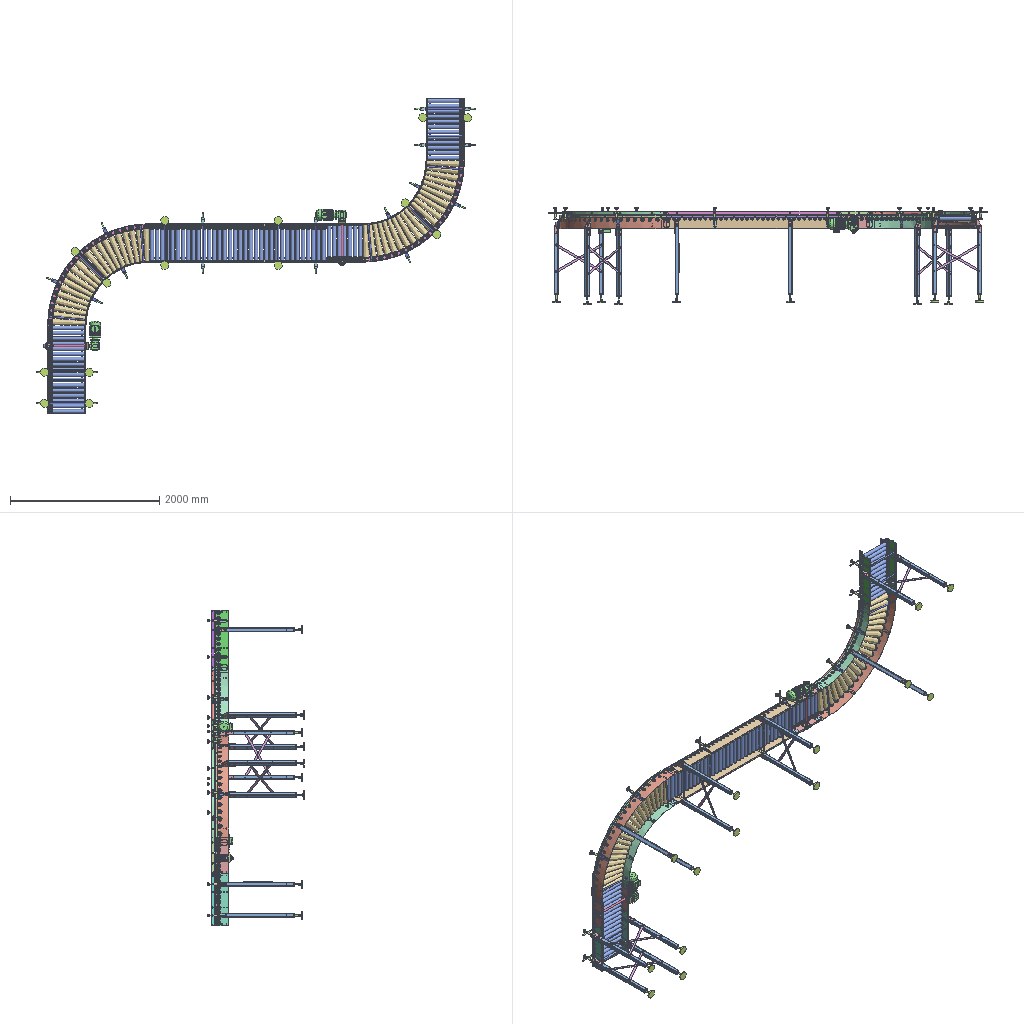Assembly | STEP file | 42 different items | 369 placed | box 5881 x 1299 x 4231 mm
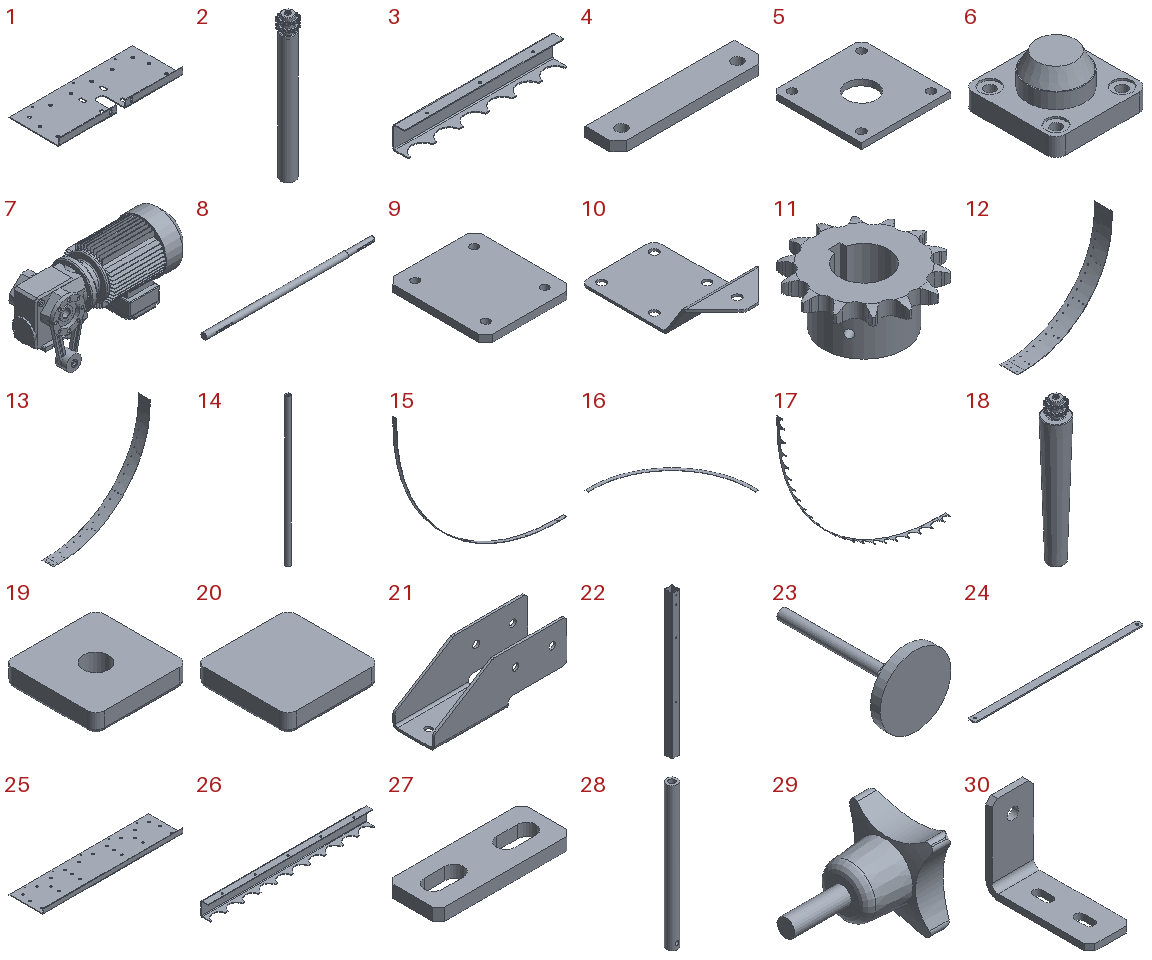Parts list (item | name | quantity | parent item | size | volume):
1 | cc-roller-motor section | x4 | in motor assembly | 418.8 x 170 x 25 mm | 188211 mm3
2 | 08b1-14 | x70 | in motor assembly, curverollers850, straight section rollers-09, straight section rollers-32, straight section rollers-10 | 63.262 x 61.879 x 506 mm | 1624253 mm3
3 | cc-coverrollers-05 | x2 | in motor assembly | 418.8 x 40 x 60 mm | 110529 mm3
4 | weldment back plate | x2 | in backplate weld | 90 x 20 x 6 mm | 10234 mm3
5 | backplate | x4 | in backplate weld, motor assembly | 90 x 90 x 6 mm | 42888 mm3
6 | 50502A | x4 | in motor assembly | 98 x 98 x 52 mm | 215908 mm3
7 | SA37TDT80N4 | x2 | in motor assembly | 398.5 x 155.5 x 203.5 mm | 5032005 mm3
8 | shaftfor roller511 | x2 | in motor assembly | 713 x 25 x 25 mm | 326518 mm3
9 | linkroller | x12 | in motor assembly, curverollers850 | 75 x 85 x 6 mm | 36985 mm3
10 | torque arm 110 | x2 | in motor assembly | 98 x 179 x 41 mm | 52160 mm3
11 | 08b1-14 | x2 | in motor assembly | 63.262 x 61.879 x 28 mm | 29059 mm3
12 | curverollersinside | x2 | in curverollers850 | 920 x 170 x 920 mm | 620259 mm3
13 | curverollersoutside | x2 | in curverollers850 | 1429 x 170 x 1429 mm | 959320 mm3
14 | axe506 | x14 | in curverollers850, straight section rollers-09, straight section rollers-32, straight section rollers-10 | 15 x 15 x 506 mm | 87993 mm3
15 | covercurveroller-p1 | x2 | in covercurveroller | 1431 x 30 x 1431 mm | 169835 mm3
16 | covercurveroller-p2 | x2 | in covercurveroller | 1428 x 1428 x 2.5 mm | 306725 mm3
17 | covercurveroller-p11 | x2 | in covercurveroller | 1374 x 60 x 1374 mm | 150099 mm3
18 | 08b1-14 | x42 | in curverollers850 | 83.871 x 83.871 x 506 mm | 1796791 mm3
19 | 14831 | x14 | in legfor roller | 50 x 50 x 10 mm | 23160 mm3
20 | 14831_CPY | x14 | in legfor roller | 50 x 50 x 10 mm | 24664 mm3
21 | Leg support-05 | x14 | in legfor roller | 180 x 56.5 x 70 mm | 69908 mm3
22 | 50x50xL-07 | x14 | in legfor roller | 50 x 50 x 900 mm | 334229 mm3
23 | 17367-articulated foot | x14 | in legfor roller | 110 x 207 x 110 mm | 212192 mm3
24 | link-forlegfor roller | x14 | in legfor roller | 725.486 x 30 x 5 mm | 107937 mm3
25 | cc-roller-09 | x2 | in straight section rollers-09 | 698 x 170 x 25 mm | 328733 mm3
26 | cc-coverrollers-09 | x1 | in straight section rollers-09 | 698 x 40 x 60 mm | 184215 mm3
27 | linkfor guide | x10 | in roller guides | 65 x 25 x 6 mm | 7799 mm3
28 | axe for guide1-02 | x20 | in guide support roller, guide support roller1 | 15 x 15 x 200 mm | 33907 mm3
29 | 13468 | x20 | in guide support roller, guide support roller1 | 57.035 x 37.729 x 37.729 mm | 20662 mm3
30 | support for guide | x12 | in guide support roller | 40 x 100 x 80 mm | 38119 mm3
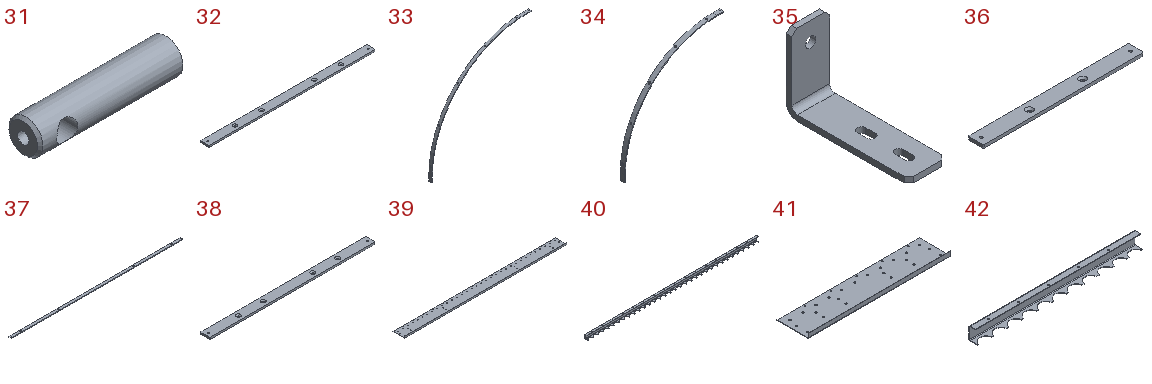31 | support1 for guide-105 | x20 | in guide support roller, guide support roller1 | 105 x 25 x 25 mm | 45078 mm3
32 | rectangular profile 40x8 | x2 | in roller guides | 767.8 x 40 x 8 mm | 241435 mm3
33 | for outer bend roller1 | x2 | in roller guides | 1382 x 40 x 1382 mm | 697130 mm3
34 | for inner bend roller | x2 | in roller guides | 938 x 40 x 938 mm | 473961 mm3
35 | support for guide1 | x8 | in guide support roller1 | 40 x 130 x 80 mm | 45319 mm3
36 | rectangular profile 40x8-419 | x4 | in roller guides | 418.8 x 40 x 8 mm | 131536 mm3
37 | rectangular profile 40x8-2303 | x2 | in roller guides | 2303 x 40 x 8 mm | 732827 mm3
38 | rectangular profile 40x8-698 | x2 | in roller guides | 698 x 40 x 8 mm | 219099 mm3
39 | cc-roller-32 | x2 | in straight section rollers-32 | 2303 x 170 x 25 mm | 1090692 mm3
40 | cc-coverrollers-32 | x1 | in straight section rollers-32 | 2303 x 40 x 60 mm | 607914 mm3
41 | cc-roller-10 | x2 | in straight section rollers-10 | 767.8 x 170 x 25 mm | 361884 mm3
42 | cc-coverrollers-10 | x1 | in straight section rollers-10 | 767.8 x 40 x 60 mm | 202679 mm3
Placements (level | parent | child | x y z in mm | rotation matrix by rows):
1 | subassembly 2 | motor assembly | -76.55 28.0 -293.364 | 1 0 0 0 1 0 0 0 1
2 | motor assembly | cc-roller-motor section | -209.4 -85.0 -12.5 | 1 0 0 0 1 0 0 0 1
2 | motor assembly | 08b1-14 | 174.5 50.0 9.104 | 1 0 0 0 -1 0 0 0 -1
2 | motor assembly | cc-roller-motor section | 209.4 -85.0 498.5 | -1 0 0 0 1 0 0 0 -1
2 | motor assembly | 08b1-14 | 104.7 50.0 9.104 | 1 0 0 0 -1 0 0 0 -1
2 | motor assembly | 08b1-14 | 34.9 50.0 9.104 | 1 0 0 0 -1 0 0 0 -1
2 | motor assembly | 08b1-14 | -34.9 50.0 9.104 | 1 0 0 0 -1 0 0 0 -1
2 | motor assembly | 08b1-14 | -104.7 50.0 9.104 | 1 0 0 0 -1 0 0 0 -1
2 | motor assembly | 08b1-14 | -174.5 50.0 9.104 | 1 0 0 0 -1 0 0 0 -1
2 | motor assembly | cc-coverrollers-05 | 209.4 65.0 -12.5 | -1 0 0 0 1 0 0 0 -1
2 | motor assembly | backplate weld | 28.767 -207.693 -38.984 | 1 0 0 0 1 0 0 0 1
3 | backplate weld | weldment back plate | -73.766 136.693 28.984 | 1 0 0 0 0 1 0 -1 0
3 | backplate weld | backplate | 126.176 142.693 28.984 | 1 0 0 0 1 0 0 0 1
2 | motor assembly | backplate | 154.943 -65.0 490.0 | 1 0 0 0 1 0 0 0 1
2 | motor assembly | 50502A | -49.0 197.629 498.5 | 1 0 0 0 1 0 0 0 1
2 | motor assembly | 50502A | 217.629 -69.0 -12.5 | 0 1 0 1 0 0 0 0 -1
2 | motor assembly | SA37TDT80N4 | -0.0 -20.0 564.5 | -1 0 0 0 0 1 0 1 -0
2 | motor assembly | shaftfor roller511 | -0.0 -20.0 653.929 | 0 0 -1 0 1 0 1 0 -0
2 | motor assembly | linkroller | -196.778 27.083 -10.0 | 1 0 0 0 1 0 0 0 1
2 | motor assembly | linkroller | -196.778 27.083 490.0 | 1 0 0 0 1 0 0 0 1
2 | motor assembly | torque arm 110 | -75.64 -116.168 498.5 | 1 0 0 0 1 0 0 0 1
2 | motor assembly | 08b1-14 | -0.0 -20.0 31.104 | 1 0 0 0 -1 0 0 0 -1
1 | subassembly 2 | curverollers850 | -123.686 119.555 202.636 | 1 0 0 0 1 0 0 0 1
2 | curverollers850 | curverollersinside | -6.975 -6.555 0.0 | 1 0 0 0 1 0 0 0 1
2 | curverollers850 | 08b1-14 | 291.536 -41.555 -486.896 | 0.3533 0.9355 0 0.9355 -0.3533 0 0 0 -1
2 | curverollers850 | 08b1-14 | 1663.433 -41.555 885.0 | 0 0 1 0 1 0 -1 0 -0
2 | curverollers850 | curverollersoutside | 142.4 -6.555 -508.5 | 1 0 0 0 1 0 0 0 1
2 | curverollers850 | axe506 | 1285.373 -146.555 -108.837 | -0.6566 -0.2625 -0.7071 0.3713 -0.9285 0 -0.6566 -0.2625 0.7071
2 | curverollers850 | axe506 | 1677.376 -146.555 731.817 | -0.02388 -0.08382 -0.9962 0.9617 -0.274 0 -0.2729 -0.9581 0.08716
2 | curverollers850 | axe506 | 444.719 -146.555 -500.84 | 0.1554 0.984 -0.08716 -0.9878 0.156 0 0.0136 0.08609 0.9962
2 | curverollers850 | covercurveroller | 1726.73 230.517 -1.54 | 0 0 -1 0 1 0 1 0 -0
3 | covercurveroller | covercurveroller-p1 | 39.985 -14.513 39.194 | 1 0 0 0 1 0 0 0 1
3 | covercurveroller | covercurveroller-p2 | 318.291 -229.571 1520.807 | 0 -1 0 0 0 1 -1 0 0
3 | covercurveroller | covercurveroller-p11 | 96.988 -44.513 96.694 | 1 0 0 0 1 0 0 0 1
2 | curverollers850 | 08b1-14 | 373.204 -58.026 -486.395 | 0.2913 -0.956 0.03489 -0.9559 -0.2923 -0.02767 0.03665 -0.02529 -0.999
2 | curverollers850 | 08b1-14 | 473.274 -58.026 -479.134 | 0.2878 -0.9514 0.1097 -0.9559 -0.2923 -0.02767 0.05839 -0.09689 -0.9936
2 | curverollers850 | 08b1-14 | 572.518 -58.026 -464.391 | 0.2826 -0.9415 0.1839 -0.9559 -0.2923 -0.02767 0.0798 -0.168 -0.9826
2 | curverollers850 | 08b1-14 | 670.377 -58.026 -442.248 | 0.2758 -0.9262 0.257 -0.9559 -0.2923 -0.02767 0.1008 -0.2381 -0.966
2 | curverollers850 | 08b1-14 | 766.3 -58.026 -412.829 | 0.2675 -0.9058 0.3287 -0.9559 -0.2923 -0.02767 0.1212 -0.3068 -0.944
2 | curverollers850 | 08b1-14 | 859.747 -58.026 -376.302 | 0.2576 -0.8802 0.3986 -0.9559 -0.2923 -0.02767 0.1409 -0.3739 -0.9167
2 | curverollers850 | 08b1-14 | 950.193 -58.026 -332.87 | 0.2463 -0.8497 0.4662 -0.9559 -0.2923 -0.02767 0.1598 -0.4388 -0.8842
2 | curverollers850 | 08b1-14 | 1037.128 -58.026 -282.78 | 0.2337 -0.8144 0.5312 -0.9559 -0.2923 -0.02767 0.1778 -0.5013 -0.8468
2 | curverollers850 | 08b1-14 | 1120.062 -58.026 -226.312 | 0.2197 -0.7745 0.5932 -0.9559 -0.2923 -0.02767 0.1948 -0.561 -0.8046
2 | curverollers850 | 08b1-14 | 1198.529 -58.026 -163.785 | 0.2045 -0.7303 0.6518 -0.9559 -0.2923 -0.02767 0.2108 -0.6175 -0.7578
2 | curverollers850 | 08b1-14 | 1272.086 -58.026 -95.55 | 0.1881 -0.6819 0.7068 -0.9559 -0.2923 -0.02767 0.2255 -0.6705 -0.7068
2 | curverollers850 | 08b1-14 | 1340.321 -58.026 -21.992 | 0.1706 -0.6297 0.7578 -0.9559 -0.2923 -0.02767 0.239 -0.7197 -0.6518
2 | curverollers850 | 08b1-14 | 1402.848 -58.026 56.474 | 0.1522 -0.574 0.8046 -0.9559 -0.2923 -0.02767 0.2511 -0.7649 -0.5932
2 | curverollers850 | 08b1-14 | 1459.316 -58.026 139.409 | 0.133 -0.515 0.8468 -0.9559 -0.2923 -0.02767 0.2618 -0.8058 -0.5312
2 | curverollers850 | 08b1-14 | 1509.407 -58.026 226.343 | 0.113 -0.4532 0.8842 -0.9559 -0.2923 -0.02767 0.271 -0.8421 -0.4662
2 | curverollers850 | 08b1-14 | 1552.838 -58.026 316.789 | 0.09234 -0.3887 0.9167 -0.9559 -0.2923 -0.02767 0.2787 -0.8737 -0.3986
2 | curverollers850 | 08b1-14 | 1589.366 -58.026 410.236 | 0.07119 -0.3221 0.944 -0.9559 -0.2923 -0.02767 0.2849 -0.9004 -0.3287
2 | curverollers850 | 08b1-14 | 1618.784 -58.026 506.159 | 0.04963 -0.2537 0.966 -0.9559 -0.2923 -0.02767 0.2894 -0.9221 -0.257
2 | curverollers850 | 08b1-14 | 1640.927 -58.026 604.018 | 0.02779 -0.1839 0.9826 -0.9559 -0.2923 -0.02767 0.2923 -0.9385 -0.1839
2 | curverollers850 | 08b1-14 | 1655.671 -58.026 703.262 | 0.005792 -0.113 0.9936 -0.9559 -0.2923 -0.02767 0.2936 -0.9496 -0.1097
2 | curverollers850 | 08b1-14 | 1662.932 -58.026 803.332 | -0.01624 -0.04146 0.999 -0.9559 -0.2923 -0.02767 0.2932 -0.9554 -0.03489
2 | curverollers850 | linkroller | 1182.536 -64.472 932.622 | 0 0 -1 0 1 0 1 0 0
2 | curverollers850 | linkroller | 1682.536 -64.472 932.622 | 0 0 -1 0 1 0 1 0 0
2 | curverollers850 | linkroller | 243.914 -168.638 -506.0 | -1 0 0 0 -1 0 0 0 1
2 | curverollers850 | linkroller | 269.159 -64.472 -6.0 | 1 0 0 0 1 0 0 0 1
1 | subassembly 2 | legfor roller | -469.367 421.023 2239.444 | 0.007492 0 1 -1 0 0.007492 0 -1 -0
2 | legfor roller | 14831 | 1367.883 487.572 1310.902 | -0.007492 0 -1 0 -1 0 -1 0 0.007492
2 | legfor roller | 14831_CPY | 450.212 487.572 1625.165 | 0.007492 0 1 0 -1 0 1 0 -0.007492
2 | legfor roller | Leg support-05 | 1845.547 603.021 1505.932 | 1 0 -0.007492 0 -1 0 -0.007492 0 -1
2 | legfor roller | 50x50xL-07 | 1359.107 636.636 1474.204 | -0.007492 0 -1 0 -1 0 -1 0 0.007492
2 | legfor roller | 17367-articulated foot | 1466.014 611.208 1463.947 | -0.007314 -1 0.001623 0.2167 0 0.9762 -0.9762 0.007492 0.2167
2 | legfor roller | Leg support-05 | 1849.375 618.895 2016.917 | 1 0 0.007492 0 1 0 -0.007492 0 1
2 | legfor roller | 14831_CPY | 454.489 764.984 2196.009 | 0 0.007492 1 1 0 0 0 1 -0.007492
2 | legfor roller | 50x50xL-07 | 1363.465 585.78 2055.931 | 0.007492 0 -1 0 1 0 1 0 0.007492
2 | legfor roller | 14831 | 1372.611 764.984 1941.852 | 0 -0.007492 -1 1 0 0 0 -1 0.007492
2 | legfor roller | 17367-articulated foot | 1470.516 611.208 2064.757 | -0.000781 -1 -0.007451 -0.9946 0 0.1042 -0.1042 0.007492 -0.9945
2 | legfor roller | link-forlegfor roller | 693.086 641.208 2075.996 | 0.4968 0.8679 0 0 0 -1 -0.8679 0.4968 -0
2 | legfor roller | link-forlegfor roller | 714.312 641.208 1448.895 | 0.5097 -0.8603 0 0 0 -1 0.8603 0.5097 -0
1 | subassembly 2 | curverollers850 | -2332.814 119.555 -303.364 | -1 0 0 0 1 0 0 0 -1
2 | curverollers850 | curverollersinside | -6.975 -6.555 0.0 | 1 0 0 0 1 0 0 0 1
2 | curverollers850 | 08b1-14 | 291.536 -41.555 -486.896 | 0.3533 0.9355 0 0.9355 -0.3533 0 0 0 -1
2 | curverollers850 | 08b1-14 | 1663.433 -41.555 885.0 | 0 0 1 0 1 0 -1 0 -0
2 | curverollers850 | curverollersoutside | 142.4 -6.555 -508.5 | 1 0 0 0 1 0 0 0 1
2 | curverollers850 | axe506 | 1285.373 -146.555 -108.837 | -0.6566 -0.2625 -0.7071 0.3713 -0.9285 0 -0.6566 -0.2625 0.7071
2 | curverollers850 | axe506 | 1677.376 -146.555 731.817 | -0.02388 -0.08382 -0.9962 0.9617 -0.274 0 -0.2729 -0.9581 0.08716
2 | curverollers850 | axe506 | 444.719 -146.555 -500.84 | 0.1554 0.984 -0.08716 -0.9878 0.156 0 0.0136 0.08609 0.9962
2 | curverollers850 | covercurveroller | 1726.73 230.517 -1.54 | 0 0 -1 0 1 0 1 0 -0
3 | covercurveroller | covercurveroller-p1 | 39.985 -14.513 39.194 | 1 0 0 0 1 0 0 0 1
3 | covercurveroller | covercurveroller-p2 | 318.291 -229.571 1520.807 | 0 -1 0 0 0 1 -1 0 0
3 | covercurveroller | covercurveroller-p11 | 96.988 -44.513 96.694 | 1 0 0 0 1 0 0 0 1
2 | curverollers850 | 08b1-14 | 373.204 -58.026 -486.395 | 0.2913 -0.956 0.03489 -0.9559 -0.2923 -0.02767 0.03665 -0.02529 -0.999
2 | curverollers850 | 08b1-14 | 473.274 -58.026 -479.134 | 0.2878 -0.9514 0.1097 -0.9559 -0.2923 -0.02767 0.05839 -0.09689 -0.9936
2 | curverollers850 | 08b1-14 | 572.518 -58.026 -464.391 | 0.2826 -0.9415 0.1839 -0.9559 -0.2923 -0.02767 0.0798 -0.168 -0.9826
2 | curverollers850 | 08b1-14 | 670.377 -58.026 -442.248 | 0.2758 -0.9262 0.257 -0.9559 -0.2923 -0.02767 0.1008 -0.2381 -0.966
2 | curverollers850 | 08b1-14 | 766.3 -58.026 -412.829 | 0.2675 -0.9058 0.3287 -0.9559 -0.2923 -0.02767 0.1212 -0.3068 -0.944
2 | curverollers850 | 08b1-14 | 859.747 -58.026 -376.302 | 0.2576 -0.8802 0.3986 -0.9559 -0.2923 -0.02767 0.1409 -0.3739 -0.9167
2 | curverollers850 | 08b1-14 | 950.193 -58.026 -332.87 | 0.2463 -0.8497 0.4662 -0.9559 -0.2923 -0.02767 0.1598 -0.4388 -0.8842
2 | curverollers850 | 08b1-14 | 1037.128 -58.026 -282.78 | 0.2337 -0.8144 0.5312 -0.9559 -0.2923 -0.02767 0.1778 -0.5013 -0.8468
2 | curverollers850 | 08b1-14 | 1120.062 -58.026 -226.312 | 0.2197 -0.7745 0.5932 -0.9559 -0.2923 -0.02767 0.1948 -0.561 -0.8046
2 | curverollers850 | 08b1-14 | 1198.529 -58.026 -163.785 | 0.2045 -0.7303 0.6518 -0.9559 -0.2923 -0.02767 0.2108 -0.6175 -0.7578
2 | curverollers850 | 08b1-14 | 1272.086 -58.026 -95.55 | 0.1881 -0.6819 0.7068 -0.9559 -0.2923 -0.02767 0.2255 -0.6705 -0.7068
2 | curverollers850 | 08b1-14 | 1340.321 -58.026 -21.992 | 0.1706 -0.6297 0.7578 -0.9559 -0.2923 -0.02767 0.239 -0.7197 -0.6518
2 | curverollers850 | 08b1-14 | 1402.848 -58.026 56.474 | 0.1522 -0.574 0.8046 -0.9559 -0.2923 -0.02767 0.2511 -0.7649 -0.5932
2 | curverollers850 | 08b1-14 | 1459.316 -58.026 139.409 | 0.133 -0.515 0.8468 -0.9559 -0.2923 -0.02767 0.2618 -0.8058 -0.5312
2 | curverollers850 | 08b1-14 | 1509.407 -58.026 226.343 | 0.113 -0.4532 0.8842 -0.9559 -0.2923 -0.02767 0.271 -0.8421 -0.4662
2 | curverollers850 | 08b1-14 | 1552.838 -58.026 316.789 | 0.09234 -0.3887 0.9167 -0.9559 -0.2923 -0.02767 0.2787 -0.8737 -0.3986
2 | curverollers850 | 08b1-14 | 1589.366 -58.026 410.236 | 0.07119 -0.3221 0.944 -0.9559 -0.2923 -0.02767 0.2849 -0.9004 -0.3287
2 | curverollers850 | 08b1-14 | 1618.784 -58.026 506.159 | 0.04963 -0.2537 0.966 -0.9559 -0.2923 -0.02767 0.2894 -0.9221 -0.257
2 | curverollers850 | 08b1-14 | 1640.927 -58.026 604.018 | 0.02779 -0.1839 0.9826 -0.9559 -0.2923 -0.02767 0.2923 -0.9385 -0.1839
2 | curverollers850 | 08b1-14 | 1655.671 -58.026 703.262 | 0.005792 -0.113 0.9936 -0.9559 -0.2923 -0.02767 0.2936 -0.9496 -0.1097
2 | curverollers850 | 08b1-14 | 1662.932 -58.026 803.332 | -0.01624 -0.04146 0.999 -0.9559 -0.2923 -0.02767 0.2932 -0.9554 -0.03489
2 | curverollers850 | linkroller | 1182.536 -64.472 932.622 | 0 0 -1 0 1 0 1 0 0
2 | curverollers850 | linkroller | 1682.536 -64.472 932.622 | 0 0 -1 0 1 0 1 0 0
2 | curverollers850 | linkroller | 243.914 -168.638 -506.0 | -1 0 0 0 -1 0 0 0 1
2 | curverollers850 | linkroller | 269.159 -64.472 -6.0 | 1 0 0 0 1 0 0 0 1
1 | subassembly 2 | motor assembly | -4005.35 28.0 -1432.764 | 0 0 1 0 1 0 -1 0 0
2 | motor assembly | cc-roller-motor section | -209.4 -85.0 -12.5 | 1 0 0 0 1 0 0 0 1
2 | motor assembly | 08b1-14 | 174.5 50.0 9.104 | 1 0 0 0 -1 0 0 0 -1
2 | motor assembly | cc-roller-motor section | 209.4 -85.0 498.5 | -1 0 0 0 1 0 0 0 -1
2 | motor assembly | 08b1-14 | 104.7 50.0 9.104 | 1 0 0 0 -1 0 0 0 -1
2 | motor assembly | 08b1-14 | 34.9 50.0 9.104 | 1 0 0 0 -1 0 0 0 -1
2 | motor assembly | 08b1-14 | -34.9 50.0 9.104 | 1 0 0 0 -1 0 0 0 -1
2 | motor assembly | 08b1-14 | -104.7 50.0 9.104 | 1 0 0 0 -1 0 0 0 -1
2 | motor assembly | 08b1-14 | -174.5 50.0 9.104 | 1 0 0 0 -1 0 0 0 -1
2 | motor assembly | cc-coverrollers-05 | 209.4 65.0 -12.5 | -1 0 0 0 1 0 0 0 -1
2 | motor assembly | backplate weld | 28.767 -207.693 -38.984 | 1 0 0 0 1 0 0 0 1
3 | backplate weld | weldment back plate | -73.766 136.693 28.984 | 1 0 0 0 0 1 0 -1 0
3 | backplate weld | backplate | 126.176 142.693 28.984 | 1 0 0 0 1 0 0 0 1
2 | motor assembly | backplate | 154.943 -65.0 490.0 | 1 0 0 0 1 0 0 0 1
2 | motor assembly | 50502A | -49.0 197.629 498.5 | 1 0 0 0 1 0 0 0 1
2 | motor assembly | 50502A | 217.629 -69.0 -12.5 | 0 1 0 1 0 0 0 0 -1
2 | motor assembly | SA37TDT80N4 | -0.0 -20.0 564.5 | -1 0 0 0 0 1 0 1 -0
2 | motor assembly | shaftfor roller511 | -0.0 -20.0 653.929 | 0 0 -1 0 1 0 1 0 -0
2 | motor assembly | linkroller | -196.778 27.083 -10.0 | 1 0 0 0 1 0 0 0 1
2 | motor assembly | linkroller | -196.778 27.083 490.0 | 1 0 0 0 1 0 0 0 1
2 | motor assembly | torque arm 110 | -75.64 -116.168 498.5 | 1 0 0 0 1 0 0 0 1
2 | motor assembly | 08b1-14 | -0.0 -20.0 31.104 | 1 0 0 0 -1 0 0 0 -1
1 | subassembly 2 | straight section rollers-09 | -4270.85 -64.5 -1634.664 | 0 0 1 0 1 0 -1 0 -0
2 | straight section rollers-09 | axe506 | 565.5 27.5 255.5 | 1 0 0 0 1 0 0 0 1
2 | straight section rollers-09 | cc-roller-09 | 7.5 7.5 253.0 | 1 0 0 0 1 0 0 0 1
2 | straight section rollers-09 | cc-coverrollers-09 | 705.5 157.5 253.0 | -1 0 0 0 1 0 0 0 -1
2 | straight section rollers-09 | cc-roller-09 | 705.5 7.5 764.0 | -1 0 0 0 1 0 0 0 -1
2 | straight section rollers-09 | 08b1-14 | 670.6 142.5 274.604 | 1 0 0 0 -1 0 0 0 -1
2 | straight section rollers-09 | 08b1-14 | 600.8 142.5 274.604 | 1 0 0 0 -1 0 0 0 -1
2 | straight section rollers-09 | 08b1-14 | 531.0 142.5 274.604 | 1 0 0 0 -1 0 0 0 -1
2 | straight section rollers-09 | 08b1-14 | 461.2 142.5 274.604 | 1 0 0 0 -1 0 0 0 -1
2 | straight section rollers-09 | 08b1-14 | 391.4 142.5 274.604 | 1 0 0 0 -1 0 0 0 -1
2 | straight section rollers-09 | 08b1-14 | 321.6 142.5 274.604 | 1 0 0 0 -1 0 0 0 -1
2 | straight section rollers-09 | 08b1-14 | 251.8 142.5 274.604 | 1 0 0 0 -1 0 0 0 -1
2 | straight section rollers-09 | 08b1-14 | 182.0 142.5 274.604 | 1 0 0 0 -1 0 0 0 -1
2 | straight section rollers-09 | 08b1-14 | 112.2 142.5 274.604 | 1 0 0 0 -1 0 0 0 -1
2 | straight section rollers-09 | 08b1-14 | 42.4 142.5 274.604 | 1 0 0 0 -1 0 0 0 -1
2 | straight section rollers-09 | axe506 | 252.0 27.5 255.5 | 1 0 0 0 1 0 0 0 1
1 | subassembly 2 | legfor roller | -1987.133 421.023 -2811.122 | -0.007492 0 -1 -1 0 0.007492 0 1 0
2 | legfor roller | 14831 | 1367.883 487.572 1310.902 | -0.007492 0 -1 0 -1 0 -1 0 0.007492
2 | legfor roller | 14831_CPY | 450.212 487.572 1625.165 | 0.007492 0 1 0 -1 0 1 0 -0.007492
2 | legfor roller | Leg support-05 | 1845.547 603.021 1505.932 | 1 0 -0.007492 0 -1 0 -0.007492 0 -1
2 | legfor roller | 50x50xL-07 | 1359.107 636.636 1474.204 | -0.007492 0 -1 0 -1 0 -1 0 0.007492
2 | legfor roller | 17367-articulated foot | 1466.014 611.208 1463.947 | -0.007314 -1 0.001623 0.2167 0 0.9762 -0.9762 0.007492 0.2167
2 | legfor roller | Leg support-05 | 1849.375 618.895 2016.917 | 1 0 0.007492 0 1 0 -0.007492 0 1
2 | legfor roller | 14831_CPY | 454.489 764.984 2196.009 | 0 0.007492 1 1 0 0 0 1 -0.007492
2 | legfor roller | 50x50xL-07 | 1363.465 585.78 2055.931 | 0.007492 0 -1 0 1 0 1 0 0.007492
2 | legfor roller | 14831 | 1372.611 764.984 1941.852 | 0 -0.007492 -1 1 0 0 0 -1 0.007492
2 | legfor roller | 17367-articulated foot | 1470.516 611.208 2064.757 | -0.000781 -1 -0.007451 -0.9946 0 0.1042 -0.1042 0.007492 -0.9945
2 | legfor roller | link-forlegfor roller | 693.086 641.208 2075.996 | 0.4968 0.8679 0 0 0 -1 -0.8679 0.4968 -0
2 | legfor roller | link-forlegfor roller | 714.312 641.208 1448.895 | 0.5097 -0.8603 0 0 0 -1 0.8603 0.5097 -0
1 | subassembly 2 | legfor roller | 1806.044 391.024 -1414.582 | -0.005298 0.7071 -0.7071 -1 0 0.007492 0.005298 0.7071 0.7071
2 | legfor roller | 14831 | 1367.883 487.572 1310.902 | -0.007492 0 -1 0 -1 0 -1 0 0.007492
2 | legfor roller | 14831_CPY | 450.212 487.572 1625.165 | 0.007492 0 1 0 -1 0 1 0 -0.007492
2 | legfor roller | Leg support-05 | 1845.547 603.021 1505.932 | 1 0 -0.007492 0 -1 0 -0.007492 0 -1
2 | legfor roller | 50x50xL-07 | 1359.107 636.636 1474.204 | -0.007492 0 -1 0 -1 0 -1 0 0.007492
2 | legfor roller | 17367-articulated foot | 1466.014 611.208 1463.947 | -0.007314 -1 0.001623 0.2167 0 0.9762 -0.9762 0.007492 0.2167
2 | legfor roller | Leg support-05 | 1849.375 618.895 2016.917 | 1 0 0.007492 0 1 0 -0.007492 0 1
2 | legfor roller | 14831_CPY | 454.489 764.984 2196.009 | 0 0.007492 1 1 0 0 0 1 -0.007492
2 | legfor roller | 50x50xL-07 | 1363.465 585.78 2055.931 | 0.007492 0 -1 0 1 0 1 0 0.007492
2 | legfor roller | 14831 | 1372.611 764.984 1941.852 | 0 -0.007492 -1 1 0 0 0 -1 0.007492
2 | legfor roller | 17367-articulated foot | 1470.516 611.208 2064.757 | -0.000781 -1 -0.007451 -0.9946 0 0.1042 -0.1042 0.007492 -0.9945
2 | legfor roller | link-forlegfor roller | 693.086 641.208 2075.996 | 0.4968 0.8679 0 0 0 -1 -0.8679 0.4968 -0
2 | legfor roller | link-forlegfor roller | 714.312 641.208 1448.895 | 0.5097 -0.8603 0 0 0 -1 0.8603 0.5097 -0
1 | subassembly 2 | legfor roller | -1542.758 421.023 -1825.58 | 0 1 0 -1 0 0.007492 0.007492 0 1
2 | legfor roller | 14831 | 1367.883 487.572 1310.902 | -0.007492 0 -1 0 -1 0 -1 0 0.007492
2 | legfor roller | 14831_CPY | 450.212 487.572 1625.165 | 0.007492 0 1 0 -1 0 1 0 -0.007492
2 | legfor roller | Leg support-05 | 1845.547 603.021 1505.932 | 1 0 -0.007492 0 -1 0 -0.007492 0 -1
2 | legfor roller | 50x50xL-07 | 1359.107 636.636 1474.204 | -0.007492 0 -1 0 -1 0 -1 0 0.007492
2 | legfor roller | 17367-articulated foot | 1466.014 611.208 1463.947 | -0.007314 -1 0.001623 0.2167 0 0.9762 -0.9762 0.007492 0.2167
2 | legfor roller | Leg support-05 | 1849.375 618.895 2016.917 | 1 0 0.007492 0 1 0 -0.007492 0 1
2 | legfor roller | 14831_CPY | 454.489 764.984 2196.009 | 0 0.007492 1 1 0 0 0 1 -0.007492
2 | legfor roller | 50x50xL-07 | 1363.465 585.78 2055.931 | 0.007492 0 -1 0 1 0 1 0 0.007492
2 | legfor roller | 14831 | 1372.611 764.984 1941.852 | 0 -0.007492 -1 1 0 0 0 -1 0.007492
2 | legfor roller | 17367-articulated foot | 1470.516 611.208 2064.757 | -0.000781 -1 -0.007451 -0.9946 0 0.1042 -0.1042 0.007492 -0.9945
2 | legfor roller | link-forlegfor roller | 693.086 641.208 2075.996 | 0.4968 0.8679 0 0 0 -1 -0.8679 0.4968 -0
2 | legfor roller | link-forlegfor roller | 714.312 641.208 1448.895 | 0.5097 -0.8603 0 0 0 -1 0.8603 0.5097 -0
1 | subassembly 2 | legfor roller | -2616.034 391.023 -2060.705 | -0.005298 0.7071 -0.7071 -1 0 0.007492 0.005298 0.7071 0.7071
2 | legfor roller | 14831 | 1367.883 487.572 1310.902 | -0.007492 0 -1 0 -1 0 -1 0 0.007492
2 | legfor roller | 14831_CPY | 450.212 487.572 1625.165 | 0.007492 0 1 0 -1 0 1 0 -0.007492
2 | legfor roller | Leg support-05 | 1845.547 603.021 1505.932 | 1 0 -0.007492 0 -1 0 -0.007492 0 -1
2 | legfor roller | 50x50xL-07 | 1359.107 636.636 1474.204 | -0.007492 0 -1 0 -1 0 -1 0 0.007492
2 | legfor roller | 17367-articulated foot | 1466.014 611.208 1463.947 | -0.007314 -1 0.001623 0.2167 0 0.9762 -0.9762 0.007492 0.2167
2 | legfor roller | Leg support-05 | 1849.375 618.895 2016.917 | 1 0 0.007492 0 1 0 -0.007492 0 1
2 | legfor roller | 14831_CPY | 454.489 764.984 2196.009 | 0 0.007492 1 1 0 0 0 1 -0.007492
2 | legfor roller | 50x50xL-07 | 1363.465 585.78 2055.931 | 0.007492 0 -1 0 1 0 1 0 0.007492
2 | legfor roller | 14831 | 1372.611 764.984 1941.852 | 0 -0.007492 -1 1 0 0 0 -1 0.007492
2 | legfor roller | 17367-articulated foot | 1470.516 611.208 2064.757 | -0.000781 -1 -0.007451 -0.9946 0 0.1042 -0.1042 0.007492 -0.9945
2 | legfor roller | link-forlegfor roller | 693.086 641.208 2075.996 | 0.4968 0.8679 0 0 0 -1 -0.8679 0.4968 -0
2 | legfor roller | link-forlegfor roller | 714.312 641.208 1448.895 | 0.5097 -0.8603 0 0 0 -1 0.8603 0.5097 -0
1 | subassembly 2 | legfor roller | -1987.133 421.023 -2393.122 | -0.007492 0 -1 -1 0 0.007492 0 1 0
2 | legfor roller | 14831 | 1367.883 487.572 1310.902 | -0.007492 0 -1 0 -1 0 -1 0 0.007492
2 | legfor roller | 14831_CPY | 450.212 487.572 1625.165 | 0.007492 0 1 0 -1 0 1 0 -0.007492
2 | legfor roller | Leg support-05 | 1845.547 603.021 1505.932 | 1 0 -0.007492 0 -1 0 -0.007492 0 -1
2 | legfor roller | 50x50xL-07 | 1359.107 636.636 1474.204 | -0.007492 0 -1 0 -1 0 -1 0 0.007492
2 | legfor roller | 17367-articulated foot | 1466.014 611.208 1463.947 | -0.007314 -1 0.001623 0.2167 0 0.9762 -0.9762 0.007492 0.2167
2 | legfor roller | Leg support-05 | 1849.375 618.895 2016.917 | 1 0 0.007492 0 1 0 -0.007492 0 1
2 | legfor roller | 14831_CPY | 454.489 764.984 2196.009 | 0 0.007492 1 1 0 0 0 1 -0.007492
2 | legfor roller | 50x50xL-07 | 1363.465 585.78 2055.931 | 0.007492 0 -1 0 1 0 1 0 0.007492
2 | legfor roller | 14831 | 1372.611 764.984 1941.852 | 0 -0.007492 -1 1 0 0 0 -1 0.007492
2 | legfor roller | 17367-articulated foot | 1470.516 611.208 2064.757 | -0.000781 -1 -0.007451 -0.9946 0 0.1042 -0.1042 0.007492 -0.9945
2 | legfor roller | link-forlegfor roller | 693.086 641.208 2075.996 | 0.4968 0.8679 0 0 0 -1 -0.8679 0.4968 -0
2 | legfor roller | link-forlegfor roller | 714.312 641.208 1448.895 | 0.5097 -0.8603 0 0 0 -1 0.8603 0.5097 -0
1 | subassembly 2 | linkfor guide | -3549.854 163.846 -931.057 | 0 0 -1 0 1 0 1 0 -0
1 | subassembly 2 | linkfor guide | -3974.846 163.846 -866.057 | 0 0 1 0 1 0 -1 0 0
1 | subassembly 2 | roller guides | -1448.011 -1380.613 425.582 | 1 0 0 0 1 0 0 0 1
2 | roller guides | guide support roller | 3085.357 1538.613 837.054 | 0 0 -1 -0.5657 -0.8246 0 -0.8246 0.5657 0
3 | guide support roller | axe for guide1-02 | 0.0 0.0 -75.0 | 1 0 0 0 1 0 0 0 1
3 | guide support roller | 13468 | -19.942 28.405 15.996 | -0.5657 0.8246 0 -0.8246 -0.5657 0 0 0 1
3 | guide support roller | support for guide | 40.212 106.981 75.996 | 0.8246 -0.5657 0 -0.5657 -0.8246 0 0 0 -1
3 | guide support roller | support1 for guide-105 | -15.089 -21.994 13.53 | 0.5657 0 0.8246 0.8246 0 -0.5657 0 1 -0
2 | roller guides | guide support roller | 3085.357 1538.613 1324.854 | 0 0 -1 -0.5657 -0.8246 0 -0.8246 0.5657 0
3 | guide support roller | axe for guide1-02 | 0.0 0.0 -75.0 | 1 0 0 0 1 0 0 0 1
3 | guide support roller | 13468 | -19.942 28.405 15.996 | -0.5657 0.8246 0 -0.8246 -0.5657 0 0 0 1
3 | guide support roller | support for guide | 40.212 106.981 75.996 | 0.8246 -0.5657 0 -0.5657 -0.8246 0 0 0 -1
3 | guide support roller | support1 for guide-105 | -15.089 -21.994 13.53 | 0.5657 0 0.8246 0.8246 0 -0.5657 0 1 -0
2 | roller guides | guide support roller | 2422.365 1538.613 1324.854 | 0 0 1 -0.5657 -0.8246 0 0.8246 -0.5657 -0
3 | guide support roller | axe for guide1-02 | 0.0 0.0 -75.0 | 1 0 0 0 1 0 0 0 1
3 | guide support roller | 13468 | -19.942 28.405 15.996 | -0.5657 0.8246 0 -0.8246 -0.5657 0 0 0 1
3 | guide support roller | support for guide | 40.212 106.981 75.996 | 0.8246 -0.5657 0 -0.5657 -0.8246 0 0 0 -1
3 | guide support roller | support1 for guide-105 | -15.089 -21.994 13.53 | 0.5657 0 0.8246 0.8246 0 -0.5657 0 1 -0
2 | roller guides | rectangular profile 40x8 | 2547.365 1772.801 1464.854 | 0 0 1 0 1 0 -1 0 -0
2 | roller guides | guide support roller | 2422.365 1538.613 837.054 | 0 0 1 -0.5657 -0.8246 0 0.8246 -0.5657 -0
3 | guide support roller | axe for guide1-02 | 0.0 0.0 -75.0 | 1 0 0 0 1 0 0 0 1
3 | guide support roller | 13468 | -19.942 28.405 15.996 | -0.5657 0.8246 0 -0.8246 -0.5657 0 0 0 1
3 | guide support roller | support for guide | 40.212 106.981 75.996 | 0.8246 -0.5657 0 -0.5657 -0.8246 0 0 0 -1
3 | guide support roller | support1 for guide-105 | -15.089 -21.994 13.53 | 0.5657 0 0.8246 0.8246 0 -0.5657 0 1 -0
2 | roller guides | rectangular profile 40x8 | 2960.357 1772.801 697.054 | 0 0 -1 0 1 0 1 0 0
2 | roller guides | for outer bend roller1 | 2969.861 1413.685 432.302 | 0 0 1 0 -1 0 1 0 -0
2 | roller guides | for inner bend roller | 2525.861 1413.685 242.01 | 0 0 1 0 -1 0 1 0 -0
2 | roller guides | guide support roller1 | 2950.956 1538.613 20.81 | -0.3485 0.2391 -0.9063 -0.5657 -0.8246 0 -0.7473 0.5127 0.4226
3 | guide support roller1 | axe for guide1-02 | -0.0 0.0 -75.0 | 1 0 0 0 1 0 0 0 1
3 | guide support roller1 | 13468 | -19.942 28.405 15.996 | -0.5657 0.8246 0 -0.8246 -0.5657 0 0 0 1
3 | guide support roller1 | support for guide1 | 40.212 106.981 75.996 | 0.8246 -0.5657 0 -0.5657 -0.8246 0 0 0 -1
3 | guide support roller1 | support1 for guide-105 | -15.089 -21.994 13.53 | 0.5657 0 0.8246 0.8246 0 -0.5657 0 1 -0
2 | roller guides | guide support roller1 | 2350.081 1538.613 301.002 | 0.3485 -0.2391 0.9063 -0.5657 -0.8246 0 0.7473 -0.5127 -0.4226
3 | guide support roller1 | axe for guide1-02 | -0.0 0.0 -75.0 | 1 0 0 0 1 0 0 0 1
3 | guide support roller1 | 13468 | -19.942 28.405 15.996 | -0.5657 0.8246 0 -0.8246 -0.5657 0 0 0 1
3 | guide support roller1 | support for guide1 | 40.212 106.981 75.996 | 0.8246 -0.5657 0 -0.5657 -0.8246 0 0 0 -1
3 | guide support roller1 | support1 for guide-105 | -15.089 -21.994 13.53 | 0.5657 0 0.8246 0.8246 0 -0.5657 0 1 -0
2 | roller guides | guide support roller1 | 1976.913 1538.613 -72.166 | 0.7473 -0.5127 0.4226 -0.5657 -0.8246 0 0.3485 -0.2391 -0.9063
3 | guide support roller1 | axe for guide1-02 | -0.0 0.0 -75.0 | 1 0 0 0 1 0 0 0 1
3 | guide support roller1 | 13468 | -19.942 28.405 15.996 | -0.5657 0.8246 0 -0.8246 -0.5657 0 0 0 1
3 | guide support roller1 | support for guide1 | 40.212 106.981 75.996 | 0.8246 -0.5657 0 -0.5657 -0.8246 0 0 0 -1
3 | guide support roller1 | support1 for guide-105 | -15.089 -21.994 13.53 | 0.5657 0 0.8246 0.8246 0 -0.5657 0 1 -0
2 | roller guides | guide support roller1 | 2257.105 1538.613 -673.041 | -0.7473 0.5127 -0.4226 -0.5657 -0.8246 0 -0.3485 0.2391 0.9063
3 | guide support roller1 | axe for guide1-02 | -0.0 0.0 -75.0 | 1 0 0 0 1 0 0 0 1
3 | guide support roller1 | 13468 | -19.942 28.405 15.996 | -0.5657 0.8246 0 -0.8246 -0.5657 0 0 0 1
3 | guide support roller1 | support for guide1 | 40.212 106.981 75.996 | 0.8246 -0.5657 0 -0.5657 -0.8246 0 0 0 -1
3 | guide support roller1 | support1 for guide-105 | -15.089 -21.994 13.53 | 0.5657 0 0.8246 0.8246 0 -0.5657 0 1 -0
2 | roller guides | linkfor guide | 1555.861 1544.459 -688.442 | 1 0 0 0 1 0 0 0 1
2 | roller guides | linkfor guide | 1555.861 1544.459 -269.45 | 1 0 0 0 1 0 0 0 1
2 | roller guides | rectangular profile 40x8-419 | 1580.861 1772.801 -269.45 | -1 0 0 0 1 0 0 0 -1
2 | roller guides | linkfor guide | 1137.061 1544.459 -688.442 | 1 0 0 0 1 0 0 0 1
2 | roller guides | rectangular profile 40x8-419 | 1162.061 1772.801 -682.442 | 1 0 0 0 1 0 0 0 1
2 | roller guides | rectangular profile 40x8-2303 | -1141.339 1772.801 -682.442 | 1 0 0 0 1 0 0 0 1
2 | roller guides | linkfor guide | 1137.061 1544.459 -269.45 | 1 0 0 0 1 0 0 0 1
2 | roller guides | rectangular profile 40x8-2303 | 1162.061 1772.801 -269.45 | -1 0 0 0 1 0 0 0 -1
2 | roller guides | guide support roller | 1022.061 1538.613 -144.451 | 0.8246 -0.5657 0 -0.5657 -0.8246 0 0 0 -1
3 | guide support roller | axe for guide1-02 | 0.0 0.0 -75.0 | 1 0 0 0 1 0 0 0 1
3 | guide support roller | 13468 | -19.942 28.405 15.996 | -0.5657 0.8246 0 -0.8246 -0.5657 0 0 0 1
3 | guide support roller | support for guide | 40.212 106.981 75.996 | 0.8246 -0.5657 0 -0.5657 -0.8246 0 0 0 -1
3 | guide support roller | support1 for guide-105 | -15.089 -21.994 13.53 | 0.5657 0 0.8246 0.8246 0 -0.5657 0 1 -0
2 | roller guides | guide support roller | 1022.061 1538.613 -807.442 | -0.8246 0.5657 0 -0.5657 -0.8246 0 0 0 1
3 | guide support roller | axe for guide1-02 | 0.0 0.0 -75.0 | 1 0 0 0 1 0 0 0 1
3 | guide support roller | 13468 | -19.942 28.405 15.996 | -0.5657 0.8246 0 -0.8246 -0.5657 0 0 0 1
3 | guide support roller | support for guide | 40.212 106.981 75.996 | 0.8246 -0.5657 0 -0.5657 -0.8246 0 0 0 -1
3 | guide support roller | support1 for guide-105 | -15.089 -21.994 13.53 | 0.5657 0 0.8246 0.8246 0 -0.5657 0 1 -0
2 | roller guides | guide support roller | -495.489 1538.613 -807.442 | -0.8246 0.5657 0 -0.5657 -0.8246 0 0 0 1
3 | guide support roller | axe for guide1-02 | 0.0 0.0 -75.0 | 1 0 0 0 1 0 0 0 1
3 | guide support roller | 13468 | -19.942 28.405 15.996 | -0.5657 0.8246 0 -0.8246 -0.5657 0 0 0 1
3 | guide support roller | support for guide | 40.212 106.981 75.996 | 0.8246 -0.5657 0 -0.5657 -0.8246 0 0 0 -1
3 | guide support roller | support1 for guide-105 | -15.089 -21.994 13.53 | 0.5657 0 0.8246 0.8246 0 -0.5657 0 1 -0
2 | roller guides | guide support roller | -495.489 1538.613 -144.451 | 0.8246 -0.5657 0 -0.5657 -0.8246 0 0 0 -1
3 | guide support roller | axe for guide1-02 | 0.0 0.0 -75.0 | 1 0 0 0 1 0 0 0 1
3 | guide support roller | 13468 | -19.942 28.405 15.996 | -0.5657 0.8246 0 -0.8246 -0.5657 0 0 0 1
3 | guide support roller | support for guide | 40.212 106.981 75.996 | 0.8246 -0.5657 0 -0.5657 -0.8246 0 0 0 -1
3 | guide support roller | support1 for guide-105 | -15.089 -21.994 13.53 | 0.5657 0 0.8246 0.8246 0 -0.5657 0 1 -0
2 | roller guides | linkfor guide | -1181.339 1544.459 -269.45 | 1 0 0 0 1 0 0 0 1
2 | roller guides | for outer bend roller1 | -1413.595 1663.541 -277.45 | 1 0 0 0 1 0 0 0 1
2 | roller guides | linkfor guide | -1181.339 1544.459 -688.442 | 1 0 0 0 1 0 0 0 1
2 | roller guides | for inner bend roller | -1564.878 1663.541 -682.442 | 1 0 0 0 1 0 0 0 1
2 | roller guides | guide support roller1 | -1537.391 1538.613 -879.726 | -0.7473 0.5127 -0.4226 -0.5657 -0.8246 0 -0.3485 0.2391 0.9063
3 | guide support roller1 | axe for guide1-02 | -0.0 0.0 -75.0 | 1 0 0 0 1 0 0 0 1
3 | guide support roller1 | 13468 | -19.942 28.405 15.996 | -0.5657 0.8246 0 -0.8246 -0.5657 0 0 0 1
3 | guide support roller1 | support for guide1 | 40.212 106.981 75.996 | 0.8246 -0.5657 0 -0.5657 -0.8246 0 0 0 -1
3 | guide support roller1 | support1 for guide-105 | -15.089 -21.994 13.53 | 0.5657 0 0.8246 0.8246 0 -0.5657 0 1 -0
2 | roller guides | guide support roller1 | -1910.559 1538.613 -1252.894 | -0.3485 0.2391 -0.9063 -0.5657 -0.8246 0 -0.7473 0.5127 0.4226
3 | guide support roller1 | axe for guide1-02 | -0.0 0.0 -75.0 | 1 0 0 0 1 0 0 0 1
3 | guide support roller1 | 13468 | -19.942 28.405 15.996 | -0.5657 0.8246 0 -0.8246 -0.5657 0 0 0 1
3 | guide support roller1 | support for guide1 | 40.212 106.981 75.996 | 0.8246 -0.5657 0 -0.5657 -0.8246 0 0 0 -1
3 | guide support roller1 | support1 for guide-105 | -15.089 -21.994 13.53 | 0.5657 0 0.8246 0.8246 0 -0.5657 0 1 -0
2 | roller guides | guide support roller1 | -1817.583 1538.613 -278.851 | 0.7473 -0.5127 0.4226 -0.5657 -0.8246 0 0.3485 -0.2391 -0.9063
3 | guide support roller1 | axe for guide1-02 | -0.0 0.0 -75.0 | 1 0 0 0 1 0 0 0 1
3 | guide support roller1 | 13468 | -19.942 28.405 15.996 | -0.5657 0.8246 0 -0.8246 -0.5657 0 0 0 1
3 | guide support roller1 | support for guide1 | 40.212 106.981 75.996 | 0.8246 -0.5657 0 -0.5657 -0.8246 0 0 0 -1
3 | guide support roller1 | support1 for guide-105 | -15.089 -21.994 13.53 | 0.5657 0 0.8246 0.8246 0 -0.5657 0 1 -0
2 | roller guides | guide support roller1 | -2511.434 1538.613 -972.702 | 0.3485 -0.2391 0.9063 -0.5657 -0.8246 0 0.7473 -0.5127 -0.4226
3 | guide support roller1 | axe for guide1-02 | -0.0 0.0 -75.0 | 1 0 0 0 1 0 0 0 1
3 | guide support roller1 | 13468 | -19.942 28.405 15.996 | -0.5657 0.8246 0 -0.8246 -0.5657 0 0 0 1
3 | guide support roller1 | support for guide1 | 40.212 106.981 75.996 | 0.8246 -0.5657 0 -0.5657 -0.8246 0 0 0 -1
3 | guide support roller1 | support1 for guide-105 | -15.089 -21.994 13.53 | 0.5657 0 0.8246 0.8246 0 -0.5657 0 1 -0
2 | roller guides | guide support roller | -2645.835 1538.613 -2625.746 | 0 0 1 -0.5657 -0.8246 0 0.8246 -0.5657 0
3 | guide support roller | axe for guide1-02 | 0.0 0.0 -75.0 | 1 0 0 0 1 0 0 0 1
3 | guide support roller | 13468 | -19.942 28.405 15.996 | -0.5657 0.8246 0 -0.8246 -0.5657 0 0 0 1
3 | guide support roller | support for guide | 40.212 106.981 75.996 | 0.8246 -0.5657 0 -0.5657 -0.8246 0 0 0 -1
3 | guide support roller | support1 for guide-105 | -15.089 -21.994 13.53 | 0.5657 0 0.8246 0.8246 0 -0.5657 0 1 -0
2 | roller guides | guide support roller | -2645.835 1538.613 -2207.746 | 0 0 1 -0.5657 -0.8246 0 0.8246 -0.5657 0
3 | guide support roller | axe for guide1-02 | 0.0 0.0 -75.0 | 1 0 0 0 1 0 0 0 1
3 | guide support roller | 13468 | -19.942 28.405 15.996 | -0.5657 0.8246 0 -0.8246 -0.5657 0 0 0 1
3 | guide support roller | support for guide | 40.212 106.981 75.996 | 0.8246 -0.5657 0 -0.5657 -0.8246 0 0 0 -1
3 | guide support roller | support1 for guide-105 | -15.089 -21.994 13.53 | 0.5657 0 0.8246 0.8246 0 -0.5657 0 1 -0
2 | roller guides | guide support roller | -1982.843 1538.613 -2625.746 | 0 0 -1 -0.5657 -0.8246 0 -0.8246 0.5657 -0
3 | guide support roller | axe for guide1-02 | 0.0 0.0 -75.0 | 1 0 0 0 1 0 0 0 1
3 | guide support roller | 13468 | -19.942 28.405 15.996 | -0.5657 0.8246 0 -0.8246 -0.5657 0 0 0 1
3 | guide support roller | support for guide | 40.212 106.981 75.996 | 0.8246 -0.5657 0 -0.5657 -0.8246 0 0 0 -1
3 | guide support roller | support1 for guide-105 | -15.089 -21.994 13.53 | 0.5657 0 0.8246 0.8246 0 -0.5657 0 1 -0
2 | roller guides | guide support roller | -1982.843 1538.613 -2207.746 | 0 0 -1 -0.5657 -0.8246 0 -0.8246 0.5657 -0
3 | guide support roller | axe for guide1-02 | 0.0 0.0 -75.0 | 1 0 0 0 1 0 0 0 1
3 | guide support roller | 13468 | -19.942 28.405 15.996 | -0.5657 0.8246 0 -0.8246 -0.5657 0 0 0 1
3 | guide support roller | support for guide | 40.212 106.981 75.996 | 0.8246 -0.5657 0 -0.5657 -0.8246 0 0 0 -1
3 | guide support roller | support1 for guide-105 | -15.089 -21.994 13.53 | 0.5657 0 0.8246 0.8246 0 -0.5657 0 1 -0
2 | roller guides | rectangular profile 40x8-698 | -2107.843 1772.801 -2765.746 | 0 0 -1 0 1 0 1 0 -0
2 | roller guides | rectangular profile 40x8-698 | -2520.835 1772.801 -2067.746 | 0 0 1 0 1 0 -1 0 0
2 | roller guides | linkfor guide | -2526.835 1544.459 -2042.746 | 0 0 1 0 1 0 -1 0 0
2 | roller guides | rectangular profile 40x8-419 | -2520.835 1772.801 -1648.946 | 0 0 1 0 1 0 -1 0 0
2 | roller guides | linkfor guide | -2101.843 1544.459 -2107.746 | 0 0 -1 0 1 0 1 0 -0
2 | roller guides | rectangular profile 40x8-419 | -2107.843 1772.801 -2067.746 | 0 0 -1 0 1 0 1 0 -0
1 | subassembly 2 | straight section rollers-32 | -278.45 -64.5 458.136 | -1 0 0 0 1 0 0 0 -1
2 | straight section rollers-32 | axe506 | 2170.9 27.5 255.5 | 1 0 0 0 1 0 0 0 1
2 | straight section rollers-32 | cc-roller-32 | 7.5 7.5 253.0 | 1 0 0 0 1 0 0 0 1
2 | straight section rollers-32 | cc-coverrollers-32 | 2310.9 157.5 253.0 | -1 0 0 0 1 0 0 0 -1
2 | straight section rollers-32 | cc-roller-32 | 2310.9 7.5 764.0 | -1 0 0 0 1 0 0 0 -1
2 | straight section rollers-32 | 08b1-14 | 2276.0 142.5 274.604 | 1 0 0 0 -1 0 0 0 -1
2 | straight section rollers-32 | 08b1-14 | 2206.2 142.5 274.604 | 1 0 0 0 -1 0 0 0 -1
2 | straight section rollers-32 | 08b1-14 | 2136.4 142.5 274.604 | 1 0 0 0 -1 0 0 0 -1
2 | straight section rollers-32 | 08b1-14 | 2066.6 142.5 274.604 | 1 0 0 0 -1 0 0 0 -1
2 | straight section rollers-32 | 08b1-14 | 1996.8 142.5 274.604 | 1 0 0 0 -1 0 0 0 -1
2 | straight section rollers-32 | 08b1-14 | 1927.0 142.5 274.604 | 1 0 0 0 -1 0 0 0 -1
2 | straight section rollers-32 | 08b1-14 | 1857.2 142.5 274.604 | 1 0 0 0 -1 0 0 0 -1
2 | straight section rollers-32 | 08b1-14 | 1787.4 142.5 274.604 | 1 0 0 0 -1 0 0 0 -1
2 | straight section rollers-32 | 08b1-14 | 1717.6 142.5 274.604 | 1 0 0 0 -1 0 0 0 -1
2 | straight section rollers-32 | 08b1-14 | 1647.8 142.5 274.604 | 1 0 0 0 -1 0 0 0 -1
2 | straight section rollers-32 | 08b1-14 | 1578.0 142.5 274.604 | 1 0 0 0 -1 0 0 0 -1
2 | straight section rollers-32 | 08b1-14 | 1508.2 142.5 274.604 | 1 0 0 0 -1 0 0 0 -1
2 | straight section rollers-32 | 08b1-14 | 1438.4 142.5 274.604 | 1 0 0 0 -1 0 0 0 -1
2 | straight section rollers-32 | 08b1-14 | 1368.6 142.5 274.604 | 1 0 0 0 -1 0 0 0 -1
2 | straight section rollers-32 | 08b1-14 | 1298.8 142.5 274.604 | 1 0 0 0 -1 0 0 0 -1
2 | straight section rollers-32 | 08b1-14 | 1229.0 142.5 274.604 | 1 0 0 0 -1 0 0 0 -1
2 | straight section rollers-32 | 08b1-14 | 1159.2 142.5 274.604 | 1 0 0 0 -1 0 0 0 -1
2 | straight section rollers-32 | 08b1-14 | 1089.4 142.5 274.604 | 1 0 0 0 -1 0 0 0 -1
2 | straight section rollers-32 | 08b1-14 | 1019.6 142.5 274.604 | 1 0 0 0 -1 0 0 0 -1
2 | straight section rollers-32 | 08b1-14 | 949.8 142.5 274.604 | 1 0 0 0 -1 0 0 0 -1
2 | straight section rollers-32 | 08b1-14 | 880.0 142.5 274.604 | 1 0 0 0 -1 0 0 0 -1
2 | straight section rollers-32 | 08b1-14 | 810.2 142.5 274.604 | 1 0 0 0 -1 0 0 0 -1
2 | straight section rollers-32 | 08b1-14 | 740.4 142.5 274.604 | 1 0 0 0 -1 0 0 0 -1
2 | straight section rollers-32 | 08b1-14 | 670.6 142.5 274.604 | 1 0 0 0 -1 0 0 0 -1
2 | straight section rollers-32 | 08b1-14 | 600.8 142.5 274.604 | 1 0 0 0 -1 0 0 0 -1
2 | straight section rollers-32 | 08b1-14 | 531.0 142.5 274.604 | 1 0 0 0 -1 0 0 0 -1
2 | straight section rollers-32 | 08b1-14 | 461.2 142.5 274.604 | 1 0 0 0 -1 0 0 0 -1
2 | straight section rollers-32 | 08b1-14 | 391.4 142.5 274.604 | 1 0 0 0 -1 0 0 0 -1
2 | straight section rollers-32 | 08b1-14 | 321.6 142.5 274.604 | 1 0 0 0 -1 0 0 0 -1
2 | straight section rollers-32 | 08b1-14 | 251.8 142.5 274.604 | 1 0 0 0 -1 0 0 0 -1
2 | straight section rollers-32 | 08b1-14 | 182.0 142.5 274.604 | 1 0 0 0 -1 0 0 0 -1
2 | straight section rollers-32 | 08b1-14 | 112.2 142.5 274.604 | 1 0 0 0 -1 0 0 0 -1
2 | straight section rollers-32 | 08b1-14 | 42.4 142.5 274.604 | 1 0 0 0 -1 0 0 0 -1
2 | straight section rollers-32 | axe506 | 147.5 27.5 255.5 | 1 0 0 0 1 0 0 0 1
2 | straight section rollers-32 | axe506 | 653.35 27.5 255.5 | 1 0 0 0 1 0 0 0 1
2 | straight section rollers-32 | axe506 | 1665.05 27.5 255.5 | 1 0 0 0 1 0 0 0 1
1 | subassembly 2 | straight section rollers-10 | 1814.35 -64.5 1115.136 | 0 0 -1 0 1 0 1 0 0
2 | straight section rollers-10 | axe506 | 635.3 27.5 255.5 | 1 0 0 0 1 0 0 0 1
2 | straight section rollers-10 | cc-roller-10 | 7.5 7.5 253.0 | 1 0 0 0 1 0 0 0 1
2 | straight section rollers-10 | cc-coverrollers-10 | 775.3 157.5 253.0 | -1 0 0 0 1 0 0 0 -1
2 | straight section rollers-10 | cc-roller-10 | 775.3 7.5 764.0 | -1 0 0 0 1 0 0 0 -1
2 | straight section rollers-10 | 08b1-14 | 740.4 142.5 274.604 | 1 0 0 0 -1 0 0 0 -1
2 | straight section rollers-10 | 08b1-14 | 670.6 142.5 274.604 | 1 0 0 0 -1 0 0 0 -1
2 | straight section rollers-10 | 08b1-14 | 600.8 142.5 274.604 | 1 0 0 0 -1 0 0 0 -1
2 | straight section rollers-10 | 08b1-14 | 531.0 142.5 274.604 | 1 0 0 0 -1 0 0 0 -1
2 | straight section rollers-10 | 08b1-14 | 461.2 142.5 274.604 | 1 0 0 0 -1 0 0 0 -1
2 | straight section rollers-10 | 08b1-14 | 391.4 142.5 274.604 | 1 0 0 0 -1 0 0 0 -1
2 | straight section rollers-10 | 08b1-14 | 321.6 142.5 274.604 | 1 0 0 0 -1 0 0 0 -1
2 | straight section rollers-10 | 08b1-14 | 251.8 142.5 274.604 | 1 0 0 0 -1 0 0 0 -1
2 | straight section rollers-10 | 08b1-14 | 182.0 142.5 274.604 | 1 0 0 0 -1 0 0 0 -1
2 | straight section rollers-10 | 08b1-14 | 112.2 142.5 274.604 | 1 0 0 0 -1 0 0 0 -1
2 | straight section rollers-10 | 08b1-14 | 42.4 142.5 274.604 | 1 0 0 0 -1 0 0 0 -1
2 | straight section rollers-10 | axe506 | 269.45 27.5 255.5 | 1 0 0 0 1 0 0 0 1
1 | subassembly 2 | legfor roller | -3060.308 421.023 -1825.58 | 0 1 0 -1 0 0.007492 0.007492 0 1
2 | legfor roller | 14831 | 1367.883 487.572 1310.902 | -0.007492 0 -1 0 -1 0 -1 0 0.007492
2 | legfor roller | 14831_CPY | 450.212 487.572 1625.165 | 0.007492 0 1 0 -1 0 1 0 -0.007492
2 | legfor roller | Leg support-05 | 1845.547 603.021 1505.932 | 1 0 -0.007492 0 -1 0 -0.007492 0 -1
2 | legfor roller | 50x50xL-07 | 1359.107 636.636 1474.204 | -0.007492 0 -1 0 -1 0 -1 0 0.007492
2 | legfor roller | 17367-articulated foot | 1466.014 611.208 1463.947 | -0.007314 -1 0.001623 0.2167 0 0.9762 -0.9762 0.007492 0.2167
2 | legfor roller | Leg support-05 | 1849.375 618.895 2016.917 | 1 0 0.007492 0 1 0 -0.007492 0 1
2 | legfor roller | 14831_CPY | 454.489 764.984 2196.009 | 0 0.007492 1 1 0 0 0 1 -0.007492
2 | legfor roller | 50x50xL-07 | 1363.465 585.78 2055.931 | 0.007492 0 -1 0 1 0 1 0 0.007492
2 | legfor roller | 14831 | 1372.611 764.984 1941.852 | 0 -0.007492 -1 1 0 0 0 -1 0.007492
2 | legfor roller | 17367-articulated foot | 1470.516 611.208 2064.757 | -0.000781 -1 -0.007451 -0.9946 0 0.1042 -0.1042 0.007492 -0.9945
2 | legfor roller | link-forlegfor roller | 693.086 641.208 2075.996 | 0.4968 0.8679 0 0 0 -1 -0.8679 0.4968 -0
2 | legfor roller | link-forlegfor roller | 714.312 641.208 1448.895 | 0.5097 -0.8603 0 0 0 -1 0.8603 0.5097 -0